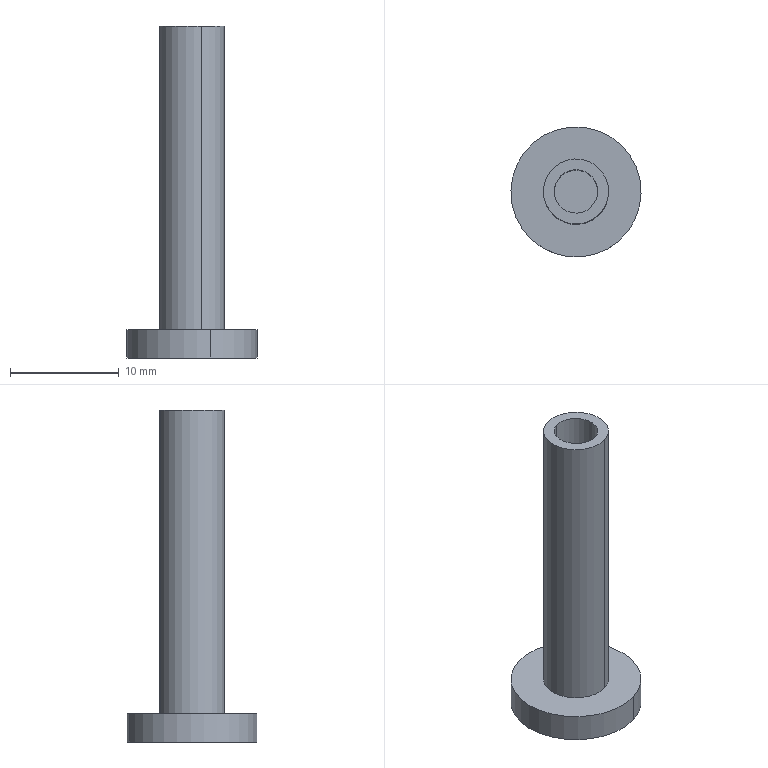Part | NX | features BREP 1 | 1 solid | 17 faces | box 12 x 12 x 30.6 mm | volume 717.248 mm3 | plane 11 | cylinder 6 | commonest cylinder face diameters 4 x2 6 x2 12 x2
STEP:
#1=CARTESIAN_POINT('',(-11.425,167.359,14.));
#2=VERTEX_POINT('',#1);
#3=CARTESIAN_POINT('',(-12.575,171.191,14.));
#4=VERTEX_POINT('',#3);
#5=CARTESIAN_POINT('',(-12.,169.275,14.));
#6=DIRECTION('',(0.,0.,1.));
#7=DIRECTION('',(-0.2874,0.9578,0.));
#8=AXIS2_PLACEMENT_3D('',#5,#6,#7);
#9=CIRCLE('',#8,2.);
#10=EDGE_CURVE('',#2,#4,#9,.T.);
#11=ORIENTED_EDGE('',*,*,#10,.T.);
#12=CARTESIAN_POINT('',(-12.575,171.191,-14.));
#13=VERTEX_POINT('',#12);
#14=CARTESIAN_POINT('',(-12.575,171.191,14.));
#15=DIRECTION('',(0.,0.,1.));
#16=VECTOR('',#15,1000.);
#17=LINE('',#14,#16);
#18=EDGE_CURVE('',#13,#4,#17,.T.);
#19=ORIENTED_EDGE('',*,*,#18,.F.);
#20=CARTESIAN_POINT('',(-11.425,167.359,-14.));
#21=VERTEX_POINT('',#20);
#22=CARTESIAN_POINT('',(-12.,169.275,-14.));
#23=DIRECTION('',(0.,0.,-1.));
#24=DIRECTION('',(-0.2874,0.9578,0.));
#25=AXIS2_PLACEMENT_3D('',#22,#23,#24);
#26=CIRCLE('',#25,2.);
#27=EDGE_CURVE('',#13,#21,#26,.T.);
#28=ORIENTED_EDGE('',*,*,#27,.T.);
#29=CARTESIAN_POINT('',(-11.425,167.359,14.));
#30=DIRECTION('',(0.,0.,-1.));
#31=VECTOR('',#30,1000.);
#32=LINE('',#29,#31);
#33=EDGE_CURVE('',#2,#21,#32,.T.);
#34=ORIENTED_EDGE('',*,*,#33,.F.);
#35=EDGE_LOOP('',(#11,#19,#28,#34));
#36=FACE_BOUND('',#35,.T.);
#37=CARTESIAN_POINT('',(-12.,169.275,14.));
#38=DIRECTION('',(0.,0.,-1.));
#39=DIRECTION('',(-0.2874,0.9578,0.));
#40=AXIS2_PLACEMENT_3D('',#37,#38,#39);
#41=CYLINDRICAL_SURFACE('',#40,2.);
#42=ADVANCED_FACE('',(#36),#41,.F.);
#43=CARTESIAN_POINT('',(-12.862,172.148,14.));
#44=VERTEX_POINT('',#43);
#45=CARTESIAN_POINT('',(-11.138,166.402,14.));
#46=VERTEX_POINT('',#45);
#47=CARTESIAN_POINT('',(-12.,169.275,14.));
#48=DIRECTION('',(0.,0.,1.));
#49=DIRECTION('',(-0.2874,0.9578,0.));
#50=AXIS2_PLACEMENT_3D('',#47,#48,#49);
#51=CIRCLE('',#50,3.);
#52=EDGE_CURVE('',#44,#46,#51,.T.);
#53=ORIENTED_EDGE('',*,*,#52,.F.);
#54=CARTESIAN_POINT('',(-12.862,172.148,-14.));
#55=VERTEX_POINT('',#54);
#56=CARTESIAN_POINT('',(-12.862,172.148,14.));
#57=DIRECTION('',(0.,0.,1.));
#58=VECTOR('',#57,1000.);
#59=LINE('',#56,#58);
#60=EDGE_CURVE('',#55,#44,#59,.T.);
#61=ORIENTED_EDGE('',*,*,#60,.F.);
#62=CARTESIAN_POINT('',(-11.138,166.402,-14.));
#63=VERTEX_POINT('',#62);
#64=CARTESIAN_POINT('',(-12.,169.275,-14.));
#65=DIRECTION('',(0.,0.,1.));
#66=DIRECTION('',(-0.2874,0.9578,0.));
#67=AXIS2_PLACEMENT_3D('',#64,#65,#66);
#68=CIRCLE('',#67,3.);
#69=EDGE_CURVE('',#55,#63,#68,.T.);
#70=ORIENTED_EDGE('',*,*,#69,.T.);
#71=CARTESIAN_POINT('',(-11.138,166.402,14.));
#72=DIRECTION('',(0.,0.,-1.));
#73=VECTOR('',#72,1000.);
#74=LINE('',#71,#73);
#75=EDGE_CURVE('',#46,#63,#74,.T.);
#76=ORIENTED_EDGE('',*,*,#75,.F.);
#77=EDGE_LOOP('',(#53,#61,#70,#76));
#78=FACE_BOUND('',#77,.T.);
#79=CARTESIAN_POINT('',(-12.,169.275,14.));
#80=DIRECTION('',(0.,0.,-1.));
#81=DIRECTION('',(-0.2874,0.9578,0.));
#82=AXIS2_PLACEMENT_3D('',#79,#80,#81);
#83=CYLINDRICAL_SURFACE('',#82,3.);
#84=ADVANCED_FACE('',(#78),#83,.T.);
#85=CARTESIAN_POINT('',(-13.725,175.022,-14.));
#86=VERTEX_POINT('',#85);
#87=CARTESIAN_POINT('',(-10.275,163.528,-14.));
#88=VERTEX_POINT('',#87);
#89=CARTESIAN_POINT('',(-12.,169.275,-14.));
#90=DIRECTION('',(0.,0.,1.));
#91=DIRECTION('',(-0.2874,0.9578,0.));
#92=AXIS2_PLACEMENT_3D('',#89,#90,#91);
#93=CIRCLE('',#92,6.);
#94=EDGE_CURVE('',#86,#88,#93,.T.);
#95=ORIENTED_EDGE('',*,*,#94,.F.);
#96=CARTESIAN_POINT('',(-13.725,175.022,-16.6));
#97=VERTEX_POINT('',#96);
#98=CARTESIAN_POINT('',(-13.725,175.022,-14.));
#99=DIRECTION('',(0.,0.,-1.));
#100=VECTOR('',#99,1000.);
#101=LINE('',#98,#100);
#102=EDGE_CURVE('',#86,#97,#101,.T.);
#103=ORIENTED_EDGE('',*,*,#102,.T.);
#104=CARTESIAN_POINT('',(-10.275,163.528,-16.6));
#105=VERTEX_POINT('',#104);
#106=CARTESIAN_POINT('',(-12.,169.275,-16.6));
#107=DIRECTION('',(0.,0.,1.));
#108=DIRECTION('',(-0.2874,0.9578,0.));
#109=AXIS2_PLACEMENT_3D('',#106,#107,#108);
#110=CIRCLE('',#109,6.);
#111=EDGE_CURVE('',#97,#105,#110,.T.);
#112=ORIENTED_EDGE('',*,*,#111,.T.);
#113=CARTESIAN_POINT('',(-10.275,163.528,-14.));
#114=DIRECTION('',(0.,0.,1.));
#115=VECTOR('',#114,1000.);
#116=LINE('',#113,#115);
#117=EDGE_CURVE('',#105,#88,#116,.T.);
#118=ORIENTED_EDGE('',*,*,#117,.T.);
#119=EDGE_LOOP('',(#95,#103,#112,#118));
#120=FACE_BOUND('',#119,.T.);
#121=CARTESIAN_POINT('',(-12.,169.275,-14.));
#122=DIRECTION('',(0.,0.,-1.));
#123=DIRECTION('',(-0.2874,0.9578,0.));
#124=AXIS2_PLACEMENT_3D('',#121,#122,#123);
#125=CYLINDRICAL_SURFACE('',#124,6.);
#126=ADVANCED_FACE('',(#120),#125,.T.);
#127=CARTESIAN_POINT('',(-12.,169.275,-16.6));
#128=DIRECTION('',(0.,0.,1.));
#129=DIRECTION('',(-0.2874,0.9578,0.));
#130=AXIS2_PLACEMENT_3D('',#127,#128,#129);
#131=CIRCLE('',#130,6.);
#132=EDGE_CURVE('',#105,#97,#131,.T.);
#133=ORIENTED_EDGE('',*,*,#132,.F.);
#134=ORIENTED_EDGE('',*,*,#111,.F.);
#135=EDGE_LOOP('',(#133,#134));
#136=FACE_BOUND('',#135,.T.);
#137=CARTESIAN_POINT('',(-11.469,171.523,-16.6));
#138=VERTEX_POINT('',#137);
#139=CARTESIAN_POINT('',(-13.681,170.859,-16.6));
#140=VERTEX_POINT('',#139);
#141=CARTESIAN_POINT('',(-12.575,171.191,-16.6));
#142=DIRECTION('',(-0.9578,-0.2874,0.));
#143=VECTOR('',#142,1000.);
#144=LINE('',#141,#143);
#145=EDGE_CURVE('',#138,#140,#144,.T.);
#146=ORIENTED_EDGE('',*,*,#145,.T.);
#147=CARTESIAN_POINT('',(-14.212,168.611,-16.6));
#148=VERTEX_POINT('',#147);
#149=CARTESIAN_POINT('',(-13.946,169.735,-16.6));
#150=DIRECTION('',(-0.23,-0.9732,0.));
#151=VECTOR('',#150,1000.);
#152=LINE('',#149,#151);
#153=EDGE_CURVE('',#140,#148,#152,.T.);
#154=ORIENTED_EDGE('',*,*,#153,.T.);
#155=CARTESIAN_POINT('',(-12.531,167.028,-16.6));
#156=VERTEX_POINT('',#155);
#157=CARTESIAN_POINT('',(-13.372,167.819,-16.6));
#158=DIRECTION('',(0.7278,-0.6858,0.));
#159=VECTOR('',#158,1000.);
#160=LINE('',#157,#159);
#161=EDGE_CURVE('',#148,#156,#160,.T.);
#162=ORIENTED_EDGE('',*,*,#161,.T.);
#163=CARTESIAN_POINT('',(-10.319,167.691,-16.6));
#164=VERTEX_POINT('',#163);
#165=CARTESIAN_POINT('',(-11.425,167.359,-16.6));
#166=DIRECTION('',(0.9578,0.2874,0.));
#167=VECTOR('',#166,1000.);
#168=LINE('',#165,#167);
#169=EDGE_CURVE('',#156,#164,#168,.T.);
#170=ORIENTED_EDGE('',*,*,#169,.T.);
#171=CARTESIAN_POINT('',(-9.788,169.939,-16.6));
#172=VERTEX_POINT('',#171);
#173=CARTESIAN_POINT('',(-10.054,168.815,-16.6));
#174=DIRECTION('',(0.23,0.9732,0.));
#175=VECTOR('',#174,1000.);
#176=LINE('',#173,#175);
#177=EDGE_CURVE('',#164,#172,#176,.T.);
#178=ORIENTED_EDGE('',*,*,#177,.T.);
#179=CARTESIAN_POINT('',(-10.628,170.731,-16.6));
#180=DIRECTION('',(-0.7278,0.6858,0.));
#181=VECTOR('',#180,1000.);
#182=LINE('',#179,#181);
#183=EDGE_CURVE('',#172,#138,#182,.T.);
#184=ORIENTED_EDGE('',*,*,#183,.T.);
#185=EDGE_LOOP('',(#146,#154,#162,#170,#178,#184));
#186=FACE_BOUND('',#185,.T.);
#187=CARTESIAN_POINT('',(-12.,169.275,-16.6));
#188=DIRECTION('',(0.,0.,1.));
#189=DIRECTION('',(0.2874,-0.9578,0.));
#190=AXIS2_PLACEMENT_3D('',#187,#188,#189);
#191=PLANE('',#190);
#192=ADVANCED_FACE('',(#136,#186),#191,.F.);
#193=ORIENTED_EDGE('',*,*,#102,.F.);
#194=CARTESIAN_POINT('',(-12.,169.275,-14.));
#195=DIRECTION('',(0.,0.,1.));
#196=DIRECTION('',(-0.2874,0.9578,0.));
#197=AXIS2_PLACEMENT_3D('',#194,#195,#196);
#198=CIRCLE('',#197,6.);
#199=EDGE_CURVE('',#88,#86,#198,.T.);
#200=ORIENTED_EDGE('',*,*,#199,.F.);
#201=ORIENTED_EDGE('',*,*,#117,.F.);
#202=ORIENTED_EDGE('',*,*,#132,.T.);
#203=EDGE_LOOP('',(#193,#200,#201,#202));
#204=FACE_BOUND('',#203,.T.);
#205=CARTESIAN_POINT('',(-12.,169.275,-14.));
#206=DIRECTION('',(0.,0.,-1.));
#207=DIRECTION('',(-0.2874,0.9578,0.));
#208=AXIS2_PLACEMENT_3D('',#205,#206,#207);
#209=CYLINDRICAL_SURFACE('',#208,6.);
#210=ADVANCED_FACE('',(#204),#209,.T.);
#211=CARTESIAN_POINT('',(-12.,169.275,-14.));
#212=DIRECTION('',(0.,0.,1.));
#213=DIRECTION('',(-0.2874,0.9578,0.));
#214=AXIS2_PLACEMENT_3D('',#211,#212,#213);
#215=CIRCLE('',#214,3.);
#216=EDGE_CURVE('',#63,#55,#215,.T.);
#217=ORIENTED_EDGE('',*,*,#216,.F.);
#218=ORIENTED_EDGE('',*,*,#69,.F.);
#219=EDGE_LOOP('',(#217,#218));
#220=FACE_BOUND('',#219,.T.);
#221=ORIENTED_EDGE('',*,*,#199,.T.);
#222=ORIENTED_EDGE('',*,*,#94,.T.);
#223=EDGE_LOOP('',(#221,#222));
#224=FACE_BOUND('',#223,.T.);
#225=CARTESIAN_POINT('',(-12.,169.275,-14.));
#226=DIRECTION('',(0.,0.,1.));
#227=DIRECTION('',(0.2874,-0.9578,0.));
#228=AXIS2_PLACEMENT_3D('',#225,#226,#227);
#229=PLANE('',#228);
#230=ADVANCED_FACE('',(#220,#224),#229,.T.);
#231=ORIENTED_EDGE('',*,*,#145,.F.);
#232=CARTESIAN_POINT('',(-11.469,171.523,-15.4));
#233=VERTEX_POINT('',#232);
#234=CARTESIAN_POINT('',(-11.469,171.523,-15.4));
#235=DIRECTION('',(0.,0.,-1.));
#236=VECTOR('',#235,1000.);
#237=LINE('',#234,#236);
#238=EDGE_CURVE('',#233,#138,#237,.T.);
#239=ORIENTED_EDGE('',*,*,#238,.F.);
#240=CARTESIAN_POINT('',(-13.681,170.859,-15.4));
#241=VERTEX_POINT('',#240);
#242=CARTESIAN_POINT('',(-12.575,171.191,-15.4));
#243=DIRECTION('',(-0.9578,-0.2874,0.));
#244=VECTOR('',#243,1000.);
#245=LINE('',#242,#244);
#246=EDGE_CURVE('',#233,#241,#245,.T.);
#247=ORIENTED_EDGE('',*,*,#246,.T.);
#248=CARTESIAN_POINT('',(-13.681,170.859,-15.4));
#249=DIRECTION('',(0.,0.,-1.));
#250=VECTOR('',#249,1000.);
#251=LINE('',#248,#250);
#252=EDGE_CURVE('',#241,#140,#251,.T.);
#253=ORIENTED_EDGE('',*,*,#252,.T.);
#254=EDGE_LOOP('',(#231,#239,#247,#253));
#255=FACE_BOUND('',#254,.T.);
#256=CARTESIAN_POINT('',(-12.575,171.191,-15.4));
#257=DIRECTION('',(0.2874,-0.9578,0.));
#258=DIRECTION('',(-0.9578,-0.2874,0.));
#259=AXIS2_PLACEMENT_3D('',#256,#257,#258);
#260=PLANE('',#259);
#261=ADVANCED_FACE('',(#255),#260,.T.);
#262=ORIENTED_EDGE('',*,*,#153,.F.);
#263=ORIENTED_EDGE('',*,*,#252,.F.);
#264=CARTESIAN_POINT('',(-14.212,168.611,-15.4));
#265=VERTEX_POINT('',#264);
#266=CARTESIAN_POINT('',(-13.946,169.735,-15.4));
#267=DIRECTION('',(-0.23,-0.9732,0.));
#268=VECTOR('',#267,1000.);
#269=LINE('',#266,#268);
#270=EDGE_CURVE('',#241,#265,#269,.T.);
#271=ORIENTED_EDGE('',*,*,#270,.T.);
#272=CARTESIAN_POINT('',(-14.212,168.611,-15.4));
#273=DIRECTION('',(0.,0.,-1.));
#274=VECTOR('',#273,1000.);
#275=LINE('',#272,#274);
#276=EDGE_CURVE('',#265,#148,#275,.T.);
#277=ORIENTED_EDGE('',*,*,#276,.T.);
#278=EDGE_LOOP('',(#262,#263,#271,#277));
#279=FACE_BOUND('',#278,.T.);
#280=CARTESIAN_POINT('',(-13.946,169.735,-15.4));
#281=DIRECTION('',(0.9732,-0.23,0.));
#282=DIRECTION('',(-0.23,-0.9732,0.));
#283=AXIS2_PLACEMENT_3D('',#280,#281,#282);
#284=PLANE('',#283);
#285=ADVANCED_FACE('',(#279),#284,.T.);
#286=ORIENTED_EDGE('',*,*,#161,.F.);
#287=ORIENTED_EDGE('',*,*,#276,.F.);
#288=CARTESIAN_POINT('',(-12.531,167.028,-15.4));
#289=VERTEX_POINT('',#288);
#290=CARTESIAN_POINT('',(-13.372,167.819,-15.4));
#291=DIRECTION('',(0.7278,-0.6858,0.));
#292=VECTOR('',#291,1000.);
#293=LINE('',#290,#292);
#294=EDGE_CURVE('',#265,#289,#293,.T.);
#295=ORIENTED_EDGE('',*,*,#294,.T.);
#296=CARTESIAN_POINT('',(-12.531,167.028,-15.4));
#297=DIRECTION('',(0.,0.,-1.));
#298=VECTOR('',#297,1000.);
#299=LINE('',#296,#298);
#300=EDGE_CURVE('',#289,#156,#299,.T.);
#301=ORIENTED_EDGE('',*,*,#300,.T.);
#302=EDGE_LOOP('',(#286,#287,#295,#301));
#303=FACE_BOUND('',#302,.T.);
#304=CARTESIAN_POINT('',(-13.372,167.819,-15.4));
#305=DIRECTION('',(0.6858,0.7278,0.));
#306=DIRECTION('',(0.7278,-0.6858,0.));
#307=AXIS2_PLACEMENT_3D('',#304,#305,#306);
#308=PLANE('',#307);
#309=ADVANCED_FACE('',(#303),#308,.T.);
#310=ORIENTED_EDGE('',*,*,#169,.F.);
#311=ORIENTED_EDGE('',*,*,#300,.F.);
#312=CARTESIAN_POINT('',(-10.319,167.691,-15.4));
#313=VERTEX_POINT('',#312);
#314=CARTESIAN_POINT('',(-11.425,167.359,-15.4));
#315=DIRECTION('',(0.9578,0.2874,0.));
#316=VECTOR('',#315,1000.);
#317=LINE('',#314,#316);
#318=EDGE_CURVE('',#289,#313,#317,.T.);
#319=ORIENTED_EDGE('',*,*,#318,.T.);
#320=CARTESIAN_POINT('',(-10.319,167.691,-15.4));
#321=DIRECTION('',(0.,0.,-1.));
#322=VECTOR('',#321,1000.);
#323=LINE('',#320,#322);
#324=EDGE_CURVE('',#313,#164,#323,.T.);
#325=ORIENTED_EDGE('',*,*,#324,.T.);
#326=EDGE_LOOP('',(#310,#311,#319,#325));
#327=FACE_BOUND('',#326,.T.);
#328=CARTESIAN_POINT('',(-11.425,167.359,-15.4));
#329=DIRECTION('',(-0.2874,0.9578,0.));
#330=DIRECTION('',(0.9578,0.2874,0.));
#331=AXIS2_PLACEMENT_3D('',#328,#329,#330);
#332=PLANE('',#331);
#333=ADVANCED_FACE('',(#327),#332,.T.);
#334=ORIENTED_EDGE('',*,*,#177,.F.);
#335=ORIENTED_EDGE('',*,*,#324,.F.);
#336=CARTESIAN_POINT('',(-9.788,169.939,-15.4));
#337=VERTEX_POINT('',#336);
#338=CARTESIAN_POINT('',(-10.054,168.815,-15.4));
#339=DIRECTION('',(0.23,0.9732,0.));
#340=VECTOR('',#339,1000.);
#341=LINE('',#338,#340);
#342=EDGE_CURVE('',#313,#337,#341,.T.);
#343=ORIENTED_EDGE('',*,*,#342,.T.);
#344=CARTESIAN_POINT('',(-9.788,169.939,-15.4));
#345=DIRECTION('',(0.,0.,-1.));
#346=VECTOR('',#345,1000.);
#347=LINE('',#344,#346);
#348=EDGE_CURVE('',#337,#172,#347,.T.);
#349=ORIENTED_EDGE('',*,*,#348,.T.);
#350=EDGE_LOOP('',(#334,#335,#343,#349));
#351=FACE_BOUND('',#350,.T.);
#352=CARTESIAN_POINT('',(-10.054,168.815,-15.4));
#353=DIRECTION('',(-0.9732,0.23,0.));
#354=DIRECTION('',(0.23,0.9732,0.));
#355=AXIS2_PLACEMENT_3D('',#352,#353,#354);
#356=PLANE('',#355);
#357=ADVANCED_FACE('',(#351),#356,.T.);
#358=ORIENTED_EDGE('',*,*,#183,.F.);
#359=ORIENTED_EDGE('',*,*,#348,.F.);
#360=CARTESIAN_POINT('',(-10.628,170.731,-15.4));
#361=DIRECTION('',(-0.7278,0.6858,0.));
#362=VECTOR('',#361,1000.);
#363=LINE('',#360,#362);
#364=EDGE_CURVE('',#337,#233,#363,.T.);
#365=ORIENTED_EDGE('',*,*,#364,.T.);
#366=ORIENTED_EDGE('',*,*,#238,.T.);
#367=EDGE_LOOP('',(#358,#359,#365,#366));
#368=FACE_BOUND('',#367,.T.);
#369=CARTESIAN_POINT('',(-10.628,170.731,-15.4));
#370=DIRECTION('',(-0.6858,-0.7278,0.));
#371=DIRECTION('',(-0.7278,0.6858,0.));
#372=AXIS2_PLACEMENT_3D('',#369,#370,#371);
#373=PLANE('',#372);
#374=ADVANCED_FACE('',(#368),#373,.T.);
#375=ORIENTED_EDGE('',*,*,#246,.F.);
#376=ORIENTED_EDGE('',*,*,#364,.F.);
#377=ORIENTED_EDGE('',*,*,#342,.F.);
#378=ORIENTED_EDGE('',*,*,#318,.F.);
#379=ORIENTED_EDGE('',*,*,#294,.F.);
#380=ORIENTED_EDGE('',*,*,#270,.F.);
#381=EDGE_LOOP('',(#375,#376,#377,#378,#379,#380));
#382=FACE_BOUND('',#381,.T.);
#383=CARTESIAN_POINT('',(-12.,169.275,-15.4));
#384=DIRECTION('',(0.,0.,1.));
#385=DIRECTION('',(0.2874,-0.9578,0.));
#386=AXIS2_PLACEMENT_3D('',#383,#384,#385);
#387=PLANE('',#386);
#388=ADVANCED_FACE('',(#382),#387,.F.);
#389=CARTESIAN_POINT('',(-12.,169.275,14.));
#390=DIRECTION('',(0.,0.,1.));
#391=DIRECTION('',(-0.2874,0.9578,0.));
#392=AXIS2_PLACEMENT_3D('',#389,#390,#391);
#393=CIRCLE('',#392,3.);
#394=EDGE_CURVE('',#46,#44,#393,.T.);
#395=ORIENTED_EDGE('',*,*,#394,.T.);
#396=ORIENTED_EDGE('',*,*,#52,.T.);
#397=EDGE_LOOP('',(#395,#396));
#398=FACE_BOUND('',#397,.T.);
#399=ORIENTED_EDGE('',*,*,#10,.F.);
#400=CARTESIAN_POINT('',(-12.,169.275,14.));
#401=DIRECTION('',(0.,0.,1.));
#402=DIRECTION('',(-0.2874,0.9578,0.));
#403=AXIS2_PLACEMENT_3D('',#400,#401,#402);
#404=CIRCLE('',#403,2.);
#405=EDGE_CURVE('',#4,#2,#404,.T.);
#406=ORIENTED_EDGE('',*,*,#405,.F.);
#407=EDGE_LOOP('',(#399,#406));
#408=FACE_BOUND('',#407,.T.);
#409=CARTESIAN_POINT('',(-12.,169.275,14.));
#410=DIRECTION('',(0.,0.,1.));
#411=DIRECTION('',(0.2874,-0.9578,0.));
#412=AXIS2_PLACEMENT_3D('',#409,#410,#411);
#413=PLANE('',#412);
#414=ADVANCED_FACE('',(#398,#408),#413,.T.);
#415=ORIENTED_EDGE('',*,*,#60,.T.);
#416=ORIENTED_EDGE('',*,*,#394,.F.);
#417=ORIENTED_EDGE('',*,*,#75,.T.);
#418=ORIENTED_EDGE('',*,*,#216,.T.);
#419=EDGE_LOOP('',(#415,#416,#417,#418));
#420=FACE_BOUND('',#419,.T.);
#421=CARTESIAN_POINT('',(-12.,169.275,14.));
#422=DIRECTION('',(0.,0.,-1.));
#423=DIRECTION('',(-0.2874,0.9578,0.));
#424=AXIS2_PLACEMENT_3D('',#421,#422,#423);
#425=CYLINDRICAL_SURFACE('',#424,3.);
#426=ADVANCED_FACE('',(#420),#425,.T.);
#427=ORIENTED_EDGE('',*,*,#18,.T.);
#428=ORIENTED_EDGE('',*,*,#405,.T.);
#429=ORIENTED_EDGE('',*,*,#33,.T.);
#430=CARTESIAN_POINT('',(-12.,169.275,-14.));
#431=DIRECTION('',(0.,0.,-1.));
#432=DIRECTION('',(-0.2874,0.9578,0.));
#433=AXIS2_PLACEMENT_3D('',#430,#431,#432);
#434=CIRCLE('',#433,2.);
#435=EDGE_CURVE('',#21,#13,#434,.T.);
#436=ORIENTED_EDGE('',*,*,#435,.T.);
#437=EDGE_LOOP('',(#427,#428,#429,#436));
#438=FACE_BOUND('',#437,.T.);
#439=CARTESIAN_POINT('',(-12.,169.275,14.));
#440=DIRECTION('',(0.,0.,-1.));
#441=DIRECTION('',(-0.2874,0.9578,0.));
#442=AXIS2_PLACEMENT_3D('',#439,#440,#441);
#443=CYLINDRICAL_SURFACE('',#442,2.);
#444=ADVANCED_FACE('',(#438),#443,.F.);
#445=ORIENTED_EDGE('',*,*,#435,.F.);
#446=ORIENTED_EDGE('',*,*,#27,.F.);
#447=EDGE_LOOP('',(#445,#446));
#448=FACE_BOUND('',#447,.T.);
#449=CARTESIAN_POINT('',(-12.,169.275,-14.));
#450=DIRECTION('',(0.,0.,1.));
#451=DIRECTION('',(0.2874,-0.9578,0.));
#452=AXIS2_PLACEMENT_3D('',#449,#450,#451);
#453=PLANE('',#452);
#454=ADVANCED_FACE('',(#448),#453,.T.);
#455=CLOSED_SHELL('',(#42,#84,#126,#192,#210,#230,#261,#285,#309,#333,#357,#374,#388,#414,#426,#444,#454));
#456=MANIFOLD_SOLID_BREP('',#455);
#457=(LENGTH_UNIT()NAMED_UNIT(*)SI_UNIT(.MILLI.,.METRE.));
#458=UNCERTAINTY_MEASURE_WITH_UNIT(LENGTH_MEASURE(0.00001),#457,'','');
#459=(NAMED_UNIT(*)PLANE_ANGLE_UNIT()SI_UNIT($,.RADIAN.));
#460=(NAMED_UNIT(*)SI_UNIT($,.STERADIAN.)SOLID_ANGLE_UNIT());
#461=(GEOMETRIC_REPRESENTATION_CONTEXT(3)GLOBAL_UNCERTAINTY_ASSIGNED_CONTEXT((#458))GLOBAL_UNIT_ASSIGNED_CONTEXT((#457,#459,#460))REPRESENTATION_CONTEXT('',''));
#462=ADVANCED_BREP_SHAPE_REPRESENTATION('',(#456),#461);